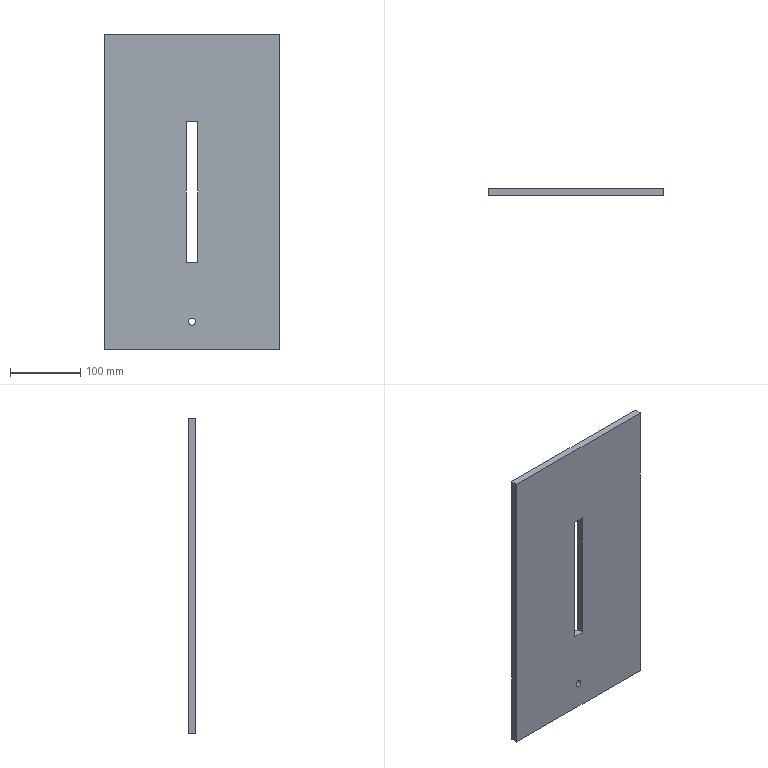Part | STEP file | tieqianjijia2 | 1 solid | 11 faces | box 250 x 10 x 450 mm | volume 1092215 mm3 | plane 10 | cylinder 1 | commonest cylinder face diameters 10 x1
STEP:
#1=CARTESIAN_POINT('',(0.,0.,0.));
#2=DIRECTION('',(0.,0.,1.));
#3=DIRECTION('',(1.,0.,0.));
#4=AXIS2_PLACEMENT_3D('',#1,#2,#3);
#5=CARTESIAN_POINT('',(0.,5.,-180.));
#6=VERTEX_POINT('',#5);
#7=CARTESIAN_POINT('',(0.,5.,-185.));
#8=DIRECTION('',(0.,1.,0.));
#9=DIRECTION('',(0.,0.,1.));
#10=AXIS2_PLACEMENT_3D('',#7,#8,#9);
#11=CIRCLE('',#10,5.);
#12=CARTESIAN_POINT('',(0.,5.,0.));
#13=DIRECTION('',(0.,1.,0.));
#14=DIRECTION('',(0.,0.,1.));
#15=AXIS2_PLACEMENT_3D('',#12,#13,#14);
#16=PLANE('',#15);
#17=CARTESIAN_POINT('',(-185.,0.));
#18=DIRECTION('',(1.,0.));
#19=AXIS2_PLACEMENT_2D('',#17,#18);
#20=CIRCLE('',#19,5.);
#21=(GEOMETRIC_REPRESENTATION_CONTEXT(2)PARAMETRIC_REPRESENTATION_CONTEXT()REPRESENTATION_CONTEXT('',''));
#22=DEFINITIONAL_REPRESENTATION('',(#20),#21);
#23=PCURVE('',#16,#22);
#24=CARTESIAN_POINT('',(0.,-5.,-185.));
#25=DIRECTION('',(0.,1.,0.));
#26=DIRECTION('',(0.,0.,1.));
#27=AXIS2_PLACEMENT_3D('',#24,#25,#26);
#28=CYLINDRICAL_SURFACE('',#27,5.);
#29=CARTESIAN_POINT('',(0.,10.));
#30=DIRECTION('',(1.,0.));
#31=VECTOR('',#30,1.);
#32=LINE('',#29,#31);
#33=(GEOMETRIC_REPRESENTATION_CONTEXT(2)PARAMETRIC_REPRESENTATION_CONTEXT()REPRESENTATION_CONTEXT('',''));
#34=DEFINITIONAL_REPRESENTATION('',(#32),#33);
#35=PCURVE('',#28,#34);
#36=SURFACE_CURVE('',#11,(#23,#35),.PCURVE_S1.);
#37=EDGE_CURVE('',#6,#6,#36,.T.);
#38=ORIENTED_EDGE('',*,*,#37,.F.);
#39=EDGE_LOOP('',(#38));
#40=FACE_BOUND('',#39,.T.);
#41=CARTESIAN_POINT('',(125.,5.,225.));
#42=VERTEX_POINT('',#41);
#43=CARTESIAN_POINT('',(125.,5.,-225.));
#44=VERTEX_POINT('',#43);
#45=CARTESIAN_POINT('',(125.,5.,-225.));
#46=DIRECTION('',(0.,0.,-1.));
#47=VECTOR('',#46,1.);
#48=LINE('',#45,#47);
#49=CARTESIAN_POINT('',(-225.,125.));
#50=DIRECTION('',(-1.,0.));
#51=VECTOR('',#50,1.);
#52=LINE('',#49,#51);
#53=(GEOMETRIC_REPRESENTATION_CONTEXT(2)PARAMETRIC_REPRESENTATION_CONTEXT()REPRESENTATION_CONTEXT('',''));
#54=DEFINITIONAL_REPRESENTATION('',(#52),#53);
#55=PCURVE('',#16,#54);
#56=CARTESIAN_POINT('',(125.,5.,-225.));
#57=DIRECTION('',(-1.,0.,0.));
#58=DIRECTION('',(0.,0.,1.));
#59=AXIS2_PLACEMENT_3D('',#56,#57,#58);
#60=PLANE('',#59);
#61=CARTESIAN_POINT('',(0.,0.));
#62=DIRECTION('',(-1.,0.));
#63=VECTOR('',#62,1.);
#64=LINE('',#61,#63);
#65=(GEOMETRIC_REPRESENTATION_CONTEXT(2)PARAMETRIC_REPRESENTATION_CONTEXT()REPRESENTATION_CONTEXT('',''));
#66=DEFINITIONAL_REPRESENTATION('',(#64),#65);
#67=PCURVE('',#60,#66);
#68=SURFACE_CURVE('',#48,(#55,#67),.PCURVE_S1.);
#69=EDGE_CURVE('',#42,#44,#68,.T.);
#70=ORIENTED_EDGE('',*,*,#69,.T.);
#71=CARTESIAN_POINT('',(-125.,5.,-225.));
#72=VERTEX_POINT('',#71);
#73=CARTESIAN_POINT('',(-125.,5.,-225.));
#74=DIRECTION('',(-1.,0.,0.));
#75=VECTOR('',#74,1.);
#76=LINE('',#73,#75);
#77=CARTESIAN_POINT('',(-225.,-125.));
#78=DIRECTION('',(0.,-1.));
#79=VECTOR('',#78,1.);
#80=LINE('',#77,#79);
#81=(GEOMETRIC_REPRESENTATION_CONTEXT(2)PARAMETRIC_REPRESENTATION_CONTEXT()REPRESENTATION_CONTEXT('',''));
#82=DEFINITIONAL_REPRESENTATION('',(#80),#81);
#83=PCURVE('',#16,#82);
#84=CARTESIAN_POINT('',(-125.,5.,-225.));
#85=DIRECTION('',(0.,0.,1.));
#86=DIRECTION('',(1.,0.,0.));
#87=AXIS2_PLACEMENT_3D('',#84,#85,#86);
#88=PLANE('',#87);
#89=CARTESIAN_POINT('',(0.,0.));
#90=DIRECTION('',(-1.,0.));
#91=VECTOR('',#90,1.);
#92=LINE('',#89,#91);
#93=(GEOMETRIC_REPRESENTATION_CONTEXT(2)PARAMETRIC_REPRESENTATION_CONTEXT()REPRESENTATION_CONTEXT('',''));
#94=DEFINITIONAL_REPRESENTATION('',(#92),#93);
#95=PCURVE('',#88,#94);
#96=SURFACE_CURVE('',#76,(#83,#95),.PCURVE_S1.);
#97=EDGE_CURVE('',#44,#72,#96,.T.);
#98=ORIENTED_EDGE('',*,*,#97,.T.);
#99=CARTESIAN_POINT('',(-125.,5.,225.));
#100=VERTEX_POINT('',#99);
#101=CARTESIAN_POINT('',(-125.,5.,-225.));
#102=DIRECTION('',(0.,0.,1.));
#103=VECTOR('',#102,1.);
#104=LINE('',#101,#103);
#105=CARTESIAN_POINT('',(-225.,-125.));
#106=DIRECTION('',(1.,0.));
#107=VECTOR('',#106,1.);
#108=LINE('',#105,#107);
#109=(GEOMETRIC_REPRESENTATION_CONTEXT(2)PARAMETRIC_REPRESENTATION_CONTEXT()REPRESENTATION_CONTEXT('',''));
#110=DEFINITIONAL_REPRESENTATION('',(#108),#109);
#111=PCURVE('',#16,#110);
#112=CARTESIAN_POINT('',(-125.,5.,-225.));
#113=DIRECTION('',(1.,0.,0.));
#114=DIRECTION('',(0.,0.,-1.));
#115=AXIS2_PLACEMENT_3D('',#112,#113,#114);
#116=PLANE('',#115);
#117=CARTESIAN_POINT('',(0.,0.));
#118=DIRECTION('',(-1.,0.));
#119=VECTOR('',#118,1.);
#120=LINE('',#117,#119);
#121=(GEOMETRIC_REPRESENTATION_CONTEXT(2)PARAMETRIC_REPRESENTATION_CONTEXT()REPRESENTATION_CONTEXT('',''));
#122=DEFINITIONAL_REPRESENTATION('',(#120),#121);
#123=PCURVE('',#116,#122);
#124=SURFACE_CURVE('',#104,(#111,#123),.PCURVE_S1.);
#125=EDGE_CURVE('',#72,#100,#124,.T.);
#126=ORIENTED_EDGE('',*,*,#125,.T.);
#127=CARTESIAN_POINT('',(-125.,5.,225.));
#128=DIRECTION('',(1.,0.,0.));
#129=VECTOR('',#128,1.);
#130=LINE('',#127,#129);
#131=CARTESIAN_POINT('',(225.,-125.));
#132=DIRECTION('',(0.,1.));
#133=VECTOR('',#132,1.);
#134=LINE('',#131,#133);
#135=(GEOMETRIC_REPRESENTATION_CONTEXT(2)PARAMETRIC_REPRESENTATION_CONTEXT()REPRESENTATION_CONTEXT('',''));
#136=DEFINITIONAL_REPRESENTATION('',(#134),#135);
#137=PCURVE('',#16,#136);
#138=CARTESIAN_POINT('',(-125.,5.,225.));
#139=DIRECTION('',(0.,0.,-1.));
#140=DIRECTION('',(-1.,0.,0.));
#141=AXIS2_PLACEMENT_3D('',#138,#139,#140);
#142=PLANE('',#141);
#143=CARTESIAN_POINT('',(0.,0.));
#144=DIRECTION('',(-1.,0.));
#145=VECTOR('',#144,1.);
#146=LINE('',#143,#145);
#147=(GEOMETRIC_REPRESENTATION_CONTEXT(2)PARAMETRIC_REPRESENTATION_CONTEXT()REPRESENTATION_CONTEXT('',''));
#148=DEFINITIONAL_REPRESENTATION('',(#146),#147);
#149=PCURVE('',#142,#148);
#150=SURFACE_CURVE('',#130,(#137,#149),.PCURVE_S1.);
#151=EDGE_CURVE('',#100,#42,#150,.T.);
#152=ORIENTED_EDGE('',*,*,#151,.T.);
#153=EDGE_LOOP('',(#70,#98,#126,#152));
#154=FACE_BOUND('',#153,.T.);
#155=CARTESIAN_POINT('',(-8.,5.,-100.));
#156=VERTEX_POINT('',#155);
#157=CARTESIAN_POINT('',(-8.,5.,100.));
#158=VERTEX_POINT('',#157);
#159=CARTESIAN_POINT('',(-8.,5.,-100.));
#160=DIRECTION('',(0.,0.,1.));
#161=VECTOR('',#160,1.);
#162=LINE('',#159,#161);
#163=CARTESIAN_POINT('',(-100.,-8.));
#164=DIRECTION('',(1.,0.));
#165=VECTOR('',#164,1.);
#166=LINE('',#163,#165);
#167=(GEOMETRIC_REPRESENTATION_CONTEXT(2)PARAMETRIC_REPRESENTATION_CONTEXT()REPRESENTATION_CONTEXT('',''));
#168=DEFINITIONAL_REPRESENTATION('',(#166),#167);
#169=PCURVE('',#16,#168);
#170=CARTESIAN_POINT('',(-8.,-5.,-100.));
#171=DIRECTION('',(-1.,0.,0.));
#172=DIRECTION('',(0.,0.,1.));
#173=AXIS2_PLACEMENT_3D('',#170,#171,#172);
#174=PLANE('',#173);
#175=CARTESIAN_POINT('',(0.,10.));
#176=DIRECTION('',(1.,0.));
#177=VECTOR('',#176,1.);
#178=LINE('',#175,#177);
#179=(GEOMETRIC_REPRESENTATION_CONTEXT(2)PARAMETRIC_REPRESENTATION_CONTEXT()REPRESENTATION_CONTEXT('',''));
#180=DEFINITIONAL_REPRESENTATION('',(#178),#179);
#181=PCURVE('',#174,#180);
#182=SURFACE_CURVE('',#162,(#169,#181),.PCURVE_S1.);
#183=EDGE_CURVE('',#156,#158,#182,.T.);
#184=ORIENTED_EDGE('',*,*,#183,.F.);
#185=CARTESIAN_POINT('',(8.,5.,-100.));
#186=VERTEX_POINT('',#185);
#187=CARTESIAN_POINT('',(-8.,5.,-100.));
#188=DIRECTION('',(1.,0.,0.));
#189=VECTOR('',#188,1.);
#190=LINE('',#187,#189);
#191=CARTESIAN_POINT('',(-100.,-8.));
#192=DIRECTION('',(0.,1.));
#193=VECTOR('',#192,1.);
#194=LINE('',#191,#193);
#195=(GEOMETRIC_REPRESENTATION_CONTEXT(2)PARAMETRIC_REPRESENTATION_CONTEXT()REPRESENTATION_CONTEXT('',''));
#196=DEFINITIONAL_REPRESENTATION('',(#194),#195);
#197=PCURVE('',#16,#196);
#198=CARTESIAN_POINT('',(-8.,-5.,-100.));
#199=DIRECTION('',(0.,0.,1.));
#200=DIRECTION('',(1.,0.,0.));
#201=AXIS2_PLACEMENT_3D('',#198,#199,#200);
#202=PLANE('',#201);
#203=CARTESIAN_POINT('',(0.,10.));
#204=DIRECTION('',(1.,0.));
#205=VECTOR('',#204,1.);
#206=LINE('',#203,#205);
#207=(GEOMETRIC_REPRESENTATION_CONTEXT(2)PARAMETRIC_REPRESENTATION_CONTEXT()REPRESENTATION_CONTEXT('',''));
#208=DEFINITIONAL_REPRESENTATION('',(#206),#207);
#209=PCURVE('',#202,#208);
#210=SURFACE_CURVE('',#190,(#197,#209),.PCURVE_S1.);
#211=EDGE_CURVE('',#156,#186,#210,.T.);
#212=ORIENTED_EDGE('',*,*,#211,.T.);
#213=CARTESIAN_POINT('',(8.,5.,100.));
#214=VERTEX_POINT('',#213);
#215=CARTESIAN_POINT('',(8.,5.,100.));
#216=DIRECTION('',(0.,0.,-1.));
#217=VECTOR('',#216,1.);
#218=LINE('',#215,#217);
#219=CARTESIAN_POINT('',(100.,8.));
#220=DIRECTION('',(-1.,0.));
#221=VECTOR('',#220,1.);
#222=LINE('',#219,#221);
#223=(GEOMETRIC_REPRESENTATION_CONTEXT(2)PARAMETRIC_REPRESENTATION_CONTEXT()REPRESENTATION_CONTEXT('',''));
#224=DEFINITIONAL_REPRESENTATION('',(#222),#223);
#225=PCURVE('',#16,#224);
#226=CARTESIAN_POINT('',(8.,-5.,100.));
#227=DIRECTION('',(1.,0.,0.));
#228=DIRECTION('',(0.,0.,-1.));
#229=AXIS2_PLACEMENT_3D('',#226,#227,#228);
#230=PLANE('',#229);
#231=CARTESIAN_POINT('',(0.,10.));
#232=DIRECTION('',(1.,0.));
#233=VECTOR('',#232,1.);
#234=LINE('',#231,#233);
#235=(GEOMETRIC_REPRESENTATION_CONTEXT(2)PARAMETRIC_REPRESENTATION_CONTEXT()REPRESENTATION_CONTEXT('',''));
#236=DEFINITIONAL_REPRESENTATION('',(#234),#235);
#237=PCURVE('',#230,#236);
#238=SURFACE_CURVE('',#218,(#225,#237),.PCURVE_S1.);
#239=EDGE_CURVE('',#214,#186,#238,.T.);
#240=ORIENTED_EDGE('',*,*,#239,.F.);
#241=CARTESIAN_POINT('',(-8.,5.,100.));
#242=DIRECTION('',(1.,0.,0.));
#243=VECTOR('',#242,1.);
#244=LINE('',#241,#243);
#245=CARTESIAN_POINT('',(100.,-8.));
#246=DIRECTION('',(0.,1.));
#247=VECTOR('',#246,1.);
#248=LINE('',#245,#247);
#249=(GEOMETRIC_REPRESENTATION_CONTEXT(2)PARAMETRIC_REPRESENTATION_CONTEXT()REPRESENTATION_CONTEXT('',''));
#250=DEFINITIONAL_REPRESENTATION('',(#248),#249);
#251=PCURVE('',#16,#250);
#252=CARTESIAN_POINT('',(-8.,-5.,100.));
#253=DIRECTION('',(0.,0.,1.));
#254=DIRECTION('',(1.,0.,0.));
#255=AXIS2_PLACEMENT_3D('',#252,#253,#254);
#256=PLANE('',#255);
#257=CARTESIAN_POINT('',(0.,10.));
#258=DIRECTION('',(1.,0.));
#259=VECTOR('',#258,1.);
#260=LINE('',#257,#259);
#261=(GEOMETRIC_REPRESENTATION_CONTEXT(2)PARAMETRIC_REPRESENTATION_CONTEXT()REPRESENTATION_CONTEXT('',''));
#262=DEFINITIONAL_REPRESENTATION('',(#260),#261);
#263=PCURVE('',#256,#262);
#264=SURFACE_CURVE('',#244,(#251,#263),.PCURVE_S1.);
#265=EDGE_CURVE('',#158,#214,#264,.T.);
#266=ORIENTED_EDGE('',*,*,#265,.F.);
#267=EDGE_LOOP('',(#184,#212,#240,#266));
#268=FACE_BOUND('',#267,.T.);
#269=ADVANCED_FACE('',(#40,#154,#268),#16,.T.);
#270=CARTESIAN_POINT('',(0.,-5.,-180.));
#271=VERTEX_POINT('',#270);
#272=CARTESIAN_POINT('',(0.,-5.,-185.));
#273=DIRECTION('',(0.,1.,0.));
#274=DIRECTION('',(0.,0.,1.));
#275=AXIS2_PLACEMENT_3D('',#272,#273,#274);
#276=CIRCLE('',#275,5.);
#277=CARTESIAN_POINT('',(0.,-5.,0.));
#278=DIRECTION('',(0.,1.,0.));
#279=DIRECTION('',(0.,0.,1.));
#280=AXIS2_PLACEMENT_3D('',#277,#278,#279);
#281=PLANE('',#280);
#282=CARTESIAN_POINT('',(-185.,0.));
#283=DIRECTION('',(1.,0.));
#284=AXIS2_PLACEMENT_2D('',#282,#283);
#285=CIRCLE('',#284,5.);
#286=(GEOMETRIC_REPRESENTATION_CONTEXT(2)PARAMETRIC_REPRESENTATION_CONTEXT()REPRESENTATION_CONTEXT('',''));
#287=DEFINITIONAL_REPRESENTATION('',(#285),#286);
#288=PCURVE('',#281,#287);
#289=CARTESIAN_POINT('',(0.,0.));
#290=DIRECTION('',(1.,0.));
#291=VECTOR('',#290,1.);
#292=LINE('',#289,#291);
#293=(GEOMETRIC_REPRESENTATION_CONTEXT(2)PARAMETRIC_REPRESENTATION_CONTEXT()REPRESENTATION_CONTEXT('',''));
#294=DEFINITIONAL_REPRESENTATION('',(#292),#293);
#295=PCURVE('',#28,#294);
#296=SURFACE_CURVE('',#276,(#288,#295),.PCURVE_S1.);
#297=EDGE_CURVE('',#271,#271,#296,.T.);
#298=ORIENTED_EDGE('',*,*,#297,.T.);
#299=EDGE_LOOP('',(#298));
#300=FACE_BOUND('',#299,.T.);
#301=CARTESIAN_POINT('',(125.,-5.,225.));
#302=VERTEX_POINT('',#301);
#303=CARTESIAN_POINT('',(125.,-5.,-225.));
#304=VERTEX_POINT('',#303);
#305=CARTESIAN_POINT('',(125.,-5.,-225.));
#306=DIRECTION('',(0.,0.,-1.));
#307=VECTOR('',#306,1.);
#308=LINE('',#305,#307);
#309=CARTESIAN_POINT('',(-225.,125.));
#310=DIRECTION('',(-1.,0.));
#311=VECTOR('',#310,1.);
#312=LINE('',#309,#311);
#313=(GEOMETRIC_REPRESENTATION_CONTEXT(2)PARAMETRIC_REPRESENTATION_CONTEXT()REPRESENTATION_CONTEXT('',''));
#314=DEFINITIONAL_REPRESENTATION('',(#312),#313);
#315=PCURVE('',#281,#314);
#316=CARTESIAN_POINT('',(0.,-10.));
#317=DIRECTION('',(-1.,0.));
#318=VECTOR('',#317,1.);
#319=LINE('',#316,#318);
#320=(GEOMETRIC_REPRESENTATION_CONTEXT(2)PARAMETRIC_REPRESENTATION_CONTEXT()REPRESENTATION_CONTEXT('',''));
#321=DEFINITIONAL_REPRESENTATION('',(#319),#320);
#322=PCURVE('',#60,#321);
#323=SURFACE_CURVE('',#308,(#315,#322),.PCURVE_S1.);
#324=EDGE_CURVE('',#302,#304,#323,.T.);
#325=ORIENTED_EDGE('',*,*,#324,.F.);
#326=CARTESIAN_POINT('',(-125.,-5.,225.));
#327=VERTEX_POINT('',#326);
#328=CARTESIAN_POINT('',(-125.,-5.,225.));
#329=DIRECTION('',(1.,0.,0.));
#330=VECTOR('',#329,1.);
#331=LINE('',#328,#330);
#332=CARTESIAN_POINT('',(225.,-125.));
#333=DIRECTION('',(0.,1.));
#334=VECTOR('',#333,1.);
#335=LINE('',#332,#334);
#336=(GEOMETRIC_REPRESENTATION_CONTEXT(2)PARAMETRIC_REPRESENTATION_CONTEXT()REPRESENTATION_CONTEXT('',''));
#337=DEFINITIONAL_REPRESENTATION('',(#335),#336);
#338=PCURVE('',#281,#337);
#339=CARTESIAN_POINT('',(0.,-10.));
#340=DIRECTION('',(-1.,0.));
#341=VECTOR('',#340,1.);
#342=LINE('',#339,#341);
#343=(GEOMETRIC_REPRESENTATION_CONTEXT(2)PARAMETRIC_REPRESENTATION_CONTEXT()REPRESENTATION_CONTEXT('',''));
#344=DEFINITIONAL_REPRESENTATION('',(#342),#343);
#345=PCURVE('',#142,#344);
#346=SURFACE_CURVE('',#331,(#338,#345),.PCURVE_S1.);
#347=EDGE_CURVE('',#327,#302,#346,.T.);
#348=ORIENTED_EDGE('',*,*,#347,.F.);
#349=CARTESIAN_POINT('',(-125.,-5.,-225.));
#350=VERTEX_POINT('',#349);
#351=CARTESIAN_POINT('',(-125.,-5.,-225.));
#352=DIRECTION('',(0.,0.,1.));
#353=VECTOR('',#352,1.);
#354=LINE('',#351,#353);
#355=CARTESIAN_POINT('',(-225.,-125.));
#356=DIRECTION('',(1.,0.));
#357=VECTOR('',#356,1.);
#358=LINE('',#355,#357);
#359=(GEOMETRIC_REPRESENTATION_CONTEXT(2)PARAMETRIC_REPRESENTATION_CONTEXT()REPRESENTATION_CONTEXT('',''));
#360=DEFINITIONAL_REPRESENTATION('',(#358),#359);
#361=PCURVE('',#281,#360);
#362=CARTESIAN_POINT('',(0.,-10.));
#363=DIRECTION('',(-1.,0.));
#364=VECTOR('',#363,1.);
#365=LINE('',#362,#364);
#366=(GEOMETRIC_REPRESENTATION_CONTEXT(2)PARAMETRIC_REPRESENTATION_CONTEXT()REPRESENTATION_CONTEXT('',''));
#367=DEFINITIONAL_REPRESENTATION('',(#365),#366);
#368=PCURVE('',#116,#367);
#369=SURFACE_CURVE('',#354,(#361,#368),.PCURVE_S1.);
#370=EDGE_CURVE('',#350,#327,#369,.T.);
#371=ORIENTED_EDGE('',*,*,#370,.F.);
#372=CARTESIAN_POINT('',(-125.,-5.,-225.));
#373=DIRECTION('',(-1.,0.,0.));
#374=VECTOR('',#373,1.);
#375=LINE('',#372,#374);
#376=CARTESIAN_POINT('',(-225.,-125.));
#377=DIRECTION('',(0.,-1.));
#378=VECTOR('',#377,1.);
#379=LINE('',#376,#378);
#380=(GEOMETRIC_REPRESENTATION_CONTEXT(2)PARAMETRIC_REPRESENTATION_CONTEXT()REPRESENTATION_CONTEXT('',''));
#381=DEFINITIONAL_REPRESENTATION('',(#379),#380);
#382=PCURVE('',#281,#381);
#383=CARTESIAN_POINT('',(0.,-10.));
#384=DIRECTION('',(-1.,0.));
#385=VECTOR('',#384,1.);
#386=LINE('',#383,#385);
#387=(GEOMETRIC_REPRESENTATION_CONTEXT(2)PARAMETRIC_REPRESENTATION_CONTEXT()REPRESENTATION_CONTEXT('',''));
#388=DEFINITIONAL_REPRESENTATION('',(#386),#387);
#389=PCURVE('',#88,#388);
#390=SURFACE_CURVE('',#375,(#382,#389),.PCURVE_S1.);
#391=EDGE_CURVE('',#304,#350,#390,.T.);
#392=ORIENTED_EDGE('',*,*,#391,.F.);
#393=EDGE_LOOP('',(#325,#348,#371,#392));
#394=FACE_BOUND('',#393,.T.);
#395=CARTESIAN_POINT('',(-8.,-5.,-100.));
#396=VERTEX_POINT('',#395);
#397=CARTESIAN_POINT('',(8.,-5.,-100.));
#398=VERTEX_POINT('',#397);
#399=CARTESIAN_POINT('',(-8.,-5.,-100.));
#400=DIRECTION('',(1.,0.,0.));
#401=VECTOR('',#400,1.);
#402=LINE('',#399,#401);
#403=CARTESIAN_POINT('',(-100.,-8.));
#404=DIRECTION('',(0.,1.));
#405=VECTOR('',#404,1.);
#406=LINE('',#403,#405);
#407=(GEOMETRIC_REPRESENTATION_CONTEXT(2)PARAMETRIC_REPRESENTATION_CONTEXT()REPRESENTATION_CONTEXT('',''));
#408=DEFINITIONAL_REPRESENTATION('',(#406),#407);
#409=PCURVE('',#281,#408);
#410=CARTESIAN_POINT('',(0.,0.));
#411=DIRECTION('',(1.,0.));
#412=VECTOR('',#411,1.);
#413=LINE('',#410,#412);
#414=(GEOMETRIC_REPRESENTATION_CONTEXT(2)PARAMETRIC_REPRESENTATION_CONTEXT()REPRESENTATION_CONTEXT('',''));
#415=DEFINITIONAL_REPRESENTATION('',(#413),#414);
#416=PCURVE('',#202,#415);
#417=SURFACE_CURVE('',#402,(#409,#416),.PCURVE_S1.);
#418=EDGE_CURVE('',#396,#398,#417,.T.);
#419=ORIENTED_EDGE('',*,*,#418,.F.);
#420=CARTESIAN_POINT('',(-8.,-5.,100.));
#421=VERTEX_POINT('',#420);
#422=CARTESIAN_POINT('',(-8.,-5.,-100.));
#423=DIRECTION('',(0.,0.,1.));
#424=VECTOR('',#423,1.);
#425=LINE('',#422,#424);
#426=CARTESIAN_POINT('',(-100.,-8.));
#427=DIRECTION('',(1.,0.));
#428=VECTOR('',#427,1.);
#429=LINE('',#426,#428);
#430=(GEOMETRIC_REPRESENTATION_CONTEXT(2)PARAMETRIC_REPRESENTATION_CONTEXT()REPRESENTATION_CONTEXT('',''));
#431=DEFINITIONAL_REPRESENTATION('',(#429),#430);
#432=PCURVE('',#281,#431);
#433=CARTESIAN_POINT('',(0.,0.));
#434=DIRECTION('',(1.,0.));
#435=VECTOR('',#434,1.);
#436=LINE('',#433,#435);
#437=(GEOMETRIC_REPRESENTATION_CONTEXT(2)PARAMETRIC_REPRESENTATION_CONTEXT()REPRESENTATION_CONTEXT('',''));
#438=DEFINITIONAL_REPRESENTATION('',(#436),#437);
#439=PCURVE('',#174,#438);
#440=SURFACE_CURVE('',#425,(#432,#439),.PCURVE_S1.);
#441=EDGE_CURVE('',#396,#421,#440,.T.);
#442=ORIENTED_EDGE('',*,*,#441,.T.);
#443=CARTESIAN_POINT('',(8.,-5.,100.));
#444=VERTEX_POINT('',#443);
#445=CARTESIAN_POINT('',(-8.,-5.,100.));
#446=DIRECTION('',(1.,0.,0.));
#447=VECTOR('',#446,1.);
#448=LINE('',#445,#447);
#449=CARTESIAN_POINT('',(100.,-8.));
#450=DIRECTION('',(0.,1.));
#451=VECTOR('',#450,1.);
#452=LINE('',#449,#451);
#453=(GEOMETRIC_REPRESENTATION_CONTEXT(2)PARAMETRIC_REPRESENTATION_CONTEXT()REPRESENTATION_CONTEXT('',''));
#454=DEFINITIONAL_REPRESENTATION('',(#452),#453);
#455=PCURVE('',#281,#454);
#456=CARTESIAN_POINT('',(0.,0.));
#457=DIRECTION('',(1.,0.));
#458=VECTOR('',#457,1.);
#459=LINE('',#456,#458);
#460=(GEOMETRIC_REPRESENTATION_CONTEXT(2)PARAMETRIC_REPRESENTATION_CONTEXT()REPRESENTATION_CONTEXT('',''));
#461=DEFINITIONAL_REPRESENTATION('',(#459),#460);
#462=PCURVE('',#256,#461);
#463=SURFACE_CURVE('',#448,(#455,#462),.PCURVE_S1.);
#464=EDGE_CURVE('',#421,#444,#463,.T.);
#465=ORIENTED_EDGE('',*,*,#464,.T.);
#466=CARTESIAN_POINT('',(8.,-5.,100.));
#467=DIRECTION('',(0.,0.,-1.));
#468=VECTOR('',#467,1.);
#469=LINE('',#466,#468);
#470=CARTESIAN_POINT('',(100.,8.));
#471=DIRECTION('',(-1.,0.));
#472=VECTOR('',#471,1.);
#473=LINE('',#470,#472);
#474=(GEOMETRIC_REPRESENTATION_CONTEXT(2)PARAMETRIC_REPRESENTATION_CONTEXT()REPRESENTATION_CONTEXT('',''));
#475=DEFINITIONAL_REPRESENTATION('',(#473),#474);
#476=PCURVE('',#281,#475);
#477=CARTESIAN_POINT('',(0.,0.));
#478=DIRECTION('',(1.,0.));
#479=VECTOR('',#478,1.);
#480=LINE('',#477,#479);
#481=(GEOMETRIC_REPRESENTATION_CONTEXT(2)PARAMETRIC_REPRESENTATION_CONTEXT()REPRESENTATION_CONTEXT('',''));
#482=DEFINITIONAL_REPRESENTATION('',(#480),#481);
#483=PCURVE('',#230,#482);
#484=SURFACE_CURVE('',#469,(#476,#483),.PCURVE_S1.);
#485=EDGE_CURVE('',#444,#398,#484,.T.);
#486=ORIENTED_EDGE('',*,*,#485,.T.);
#487=EDGE_LOOP('',(#419,#442,#465,#486));
#488=FACE_BOUND('',#487,.T.);
#489=ADVANCED_FACE('',(#300,#394,#488),#281,.F.);
#490=ORIENTED_EDGE('',*,*,#324,.T.);
#491=CARTESIAN_POINT('',(125.,5.,-225.));
#492=DIRECTION('',(0.,-1.,0.));
#493=VECTOR('',#492,1.);
#494=LINE('',#491,#493);
#495=CARTESIAN_POINT('',(0.,0.));
#496=DIRECTION('',(0.,-1.));
#497=VECTOR('',#496,1.);
#498=LINE('',#495,#497);
#499=(GEOMETRIC_REPRESENTATION_CONTEXT(2)PARAMETRIC_REPRESENTATION_CONTEXT()REPRESENTATION_CONTEXT('',''));
#500=DEFINITIONAL_REPRESENTATION('',(#498),#499);
#501=PCURVE('',#60,#500);
#502=CARTESIAN_POINT('',(250.,0.));
#503=DIRECTION('',(0.,-1.));
#504=VECTOR('',#503,1.);
#505=LINE('',#502,#504);
#506=(GEOMETRIC_REPRESENTATION_CONTEXT(2)PARAMETRIC_REPRESENTATION_CONTEXT()REPRESENTATION_CONTEXT('',''));
#507=DEFINITIONAL_REPRESENTATION('',(#505),#506);
#508=PCURVE('',#88,#507);
#509=SURFACE_CURVE('',#494,(#501,#508),.PCURVE_S1.);
#510=EDGE_CURVE('',#44,#304,#509,.T.);
#511=ORIENTED_EDGE('',*,*,#510,.F.);
#512=ORIENTED_EDGE('',*,*,#69,.F.);
#513=CARTESIAN_POINT('',(125.,5.,225.));
#514=DIRECTION('',(0.,-1.,0.));
#515=VECTOR('',#514,1.);
#516=LINE('',#513,#515);
#517=CARTESIAN_POINT('',(450.,0.));
#518=DIRECTION('',(0.,-1.));
#519=VECTOR('',#518,1.);
#520=LINE('',#517,#519);
#521=(GEOMETRIC_REPRESENTATION_CONTEXT(2)PARAMETRIC_REPRESENTATION_CONTEXT()REPRESENTATION_CONTEXT('',''));
#522=DEFINITIONAL_REPRESENTATION('',(#520),#521);
#523=PCURVE('',#60,#522);
#524=CARTESIAN_POINT('',(-250.,0.));
#525=DIRECTION('',(0.,-1.));
#526=VECTOR('',#525,1.);
#527=LINE('',#524,#526);
#528=(GEOMETRIC_REPRESENTATION_CONTEXT(2)PARAMETRIC_REPRESENTATION_CONTEXT()REPRESENTATION_CONTEXT('',''));
#529=DEFINITIONAL_REPRESENTATION('',(#527),#528);
#530=PCURVE('',#142,#529);
#531=SURFACE_CURVE('',#516,(#523,#530),.PCURVE_S1.);
#532=EDGE_CURVE('',#42,#302,#531,.T.);
#533=ORIENTED_EDGE('',*,*,#532,.T.);
#534=EDGE_LOOP('',(#490,#511,#512,#533));
#535=FACE_BOUND('',#534,.T.);
#536=ADVANCED_FACE('',(#535),#60,.F.);
#537=ORIENTED_EDGE('',*,*,#391,.T.);
#538=CARTESIAN_POINT('',(-125.,5.,-225.));
#539=DIRECTION('',(0.,-1.,0.));
#540=VECTOR('',#539,1.);
#541=LINE('',#538,#540);
#542=CARTESIAN_POINT('',(0.,0.));
#543=DIRECTION('',(0.,-1.));
#544=VECTOR('',#543,1.);
#545=LINE('',#542,#544);
#546=(GEOMETRIC_REPRESENTATION_CONTEXT(2)PARAMETRIC_REPRESENTATION_CONTEXT()REPRESENTATION_CONTEXT('',''));
#547=DEFINITIONAL_REPRESENTATION('',(#545),#546);
#548=PCURVE('',#88,#547);
#549=CARTESIAN_POINT('',(0.,0.));
#550=DIRECTION('',(0.,-1.));
#551=VECTOR('',#550,1.);
#552=LINE('',#549,#551);
#553=(GEOMETRIC_REPRESENTATION_CONTEXT(2)PARAMETRIC_REPRESENTATION_CONTEXT()REPRESENTATION_CONTEXT('',''));
#554=DEFINITIONAL_REPRESENTATION('',(#552),#553);
#555=PCURVE('',#116,#554);
#556=SURFACE_CURVE('',#541,(#548,#555),.PCURVE_S1.);
#557=EDGE_CURVE('',#72,#350,#556,.T.);
#558=ORIENTED_EDGE('',*,*,#557,.F.);
#559=ORIENTED_EDGE('',*,*,#97,.F.);
#560=ORIENTED_EDGE('',*,*,#510,.T.);
#561=EDGE_LOOP('',(#537,#558,#559,#560));
#562=FACE_BOUND('',#561,.T.);
#563=ADVANCED_FACE('',(#562),#88,.F.);
#564=ORIENTED_EDGE('',*,*,#370,.T.);
#565=CARTESIAN_POINT('',(-125.,5.,225.));
#566=DIRECTION('',(0.,-1.,0.));
#567=VECTOR('',#566,1.);
#568=LINE('',#565,#567);
#569=CARTESIAN_POINT('',(-450.,0.));
#570=DIRECTION('',(0.,-1.));
#571=VECTOR('',#570,1.);
#572=LINE('',#569,#571);
#573=(GEOMETRIC_REPRESENTATION_CONTEXT(2)PARAMETRIC_REPRESENTATION_CONTEXT()REPRESENTATION_CONTEXT('',''));
#574=DEFINITIONAL_REPRESENTATION('',(#572),#573);
#575=PCURVE('',#116,#574);
#576=CARTESIAN_POINT('',(0.,0.));
#577=DIRECTION('',(0.,-1.));
#578=VECTOR('',#577,1.);
#579=LINE('',#576,#578);
#580=(GEOMETRIC_REPRESENTATION_CONTEXT(2)PARAMETRIC_REPRESENTATION_CONTEXT()REPRESENTATION_CONTEXT('',''));
#581=DEFINITIONAL_REPRESENTATION('',(#579),#580);
#582=PCURVE('',#142,#581);
#583=SURFACE_CURVE('',#568,(#575,#582),.PCURVE_S1.);
#584=EDGE_CURVE('',#100,#327,#583,.T.);
#585=ORIENTED_EDGE('',*,*,#584,.F.);
#586=ORIENTED_EDGE('',*,*,#125,.F.);
#587=ORIENTED_EDGE('',*,*,#557,.T.);
#588=EDGE_LOOP('',(#564,#585,#586,#587));
#589=FACE_BOUND('',#588,.T.);
#590=ADVANCED_FACE('',(#589),#116,.F.);
#591=ORIENTED_EDGE('',*,*,#347,.T.);
#592=ORIENTED_EDGE('',*,*,#532,.F.);
#593=ORIENTED_EDGE('',*,*,#151,.F.);
#594=ORIENTED_EDGE('',*,*,#584,.T.);
#595=EDGE_LOOP('',(#591,#592,#593,#594));
#596=FACE_BOUND('',#595,.T.);
#597=ADVANCED_FACE('',(#596),#142,.F.);
#598=ORIENTED_EDGE('',*,*,#211,.F.);
#599=CARTESIAN_POINT('',(-8.,-5.,-100.));
#600=DIRECTION('',(0.,1.,0.));
#601=VECTOR('',#600,1.);
#602=LINE('',#599,#601);
#603=CARTESIAN_POINT('',(0.,0.));
#604=DIRECTION('',(0.,1.));
#605=VECTOR('',#604,1.);
#606=LINE('',#603,#605);
#607=(GEOMETRIC_REPRESENTATION_CONTEXT(2)PARAMETRIC_REPRESENTATION_CONTEXT()REPRESENTATION_CONTEXT('',''));
#608=DEFINITIONAL_REPRESENTATION('',(#606),#607);
#609=PCURVE('',#202,#608);
#610=CARTESIAN_POINT('',(0.,0.));
#611=DIRECTION('',(0.,1.));
#612=VECTOR('',#611,1.);
#613=LINE('',#610,#612);
#614=(GEOMETRIC_REPRESENTATION_CONTEXT(2)PARAMETRIC_REPRESENTATION_CONTEXT()REPRESENTATION_CONTEXT('',''));
#615=DEFINITIONAL_REPRESENTATION('',(#613),#614);
#616=PCURVE('',#174,#615);
#617=SURFACE_CURVE('',#602,(#609,#616),.PCURVE_S1.);
#618=EDGE_CURVE('',#396,#156,#617,.T.);
#619=ORIENTED_EDGE('',*,*,#618,.F.);
#620=ORIENTED_EDGE('',*,*,#418,.T.);
#621=CARTESIAN_POINT('',(8.,-5.,-100.));
#622=DIRECTION('',(0.,1.,0.));
#623=VECTOR('',#622,1.);
#624=LINE('',#621,#623);
#625=CARTESIAN_POINT('',(16.,0.));
#626=DIRECTION('',(0.,1.));
#627=VECTOR('',#626,1.);
#628=LINE('',#625,#627);
#629=(GEOMETRIC_REPRESENTATION_CONTEXT(2)PARAMETRIC_REPRESENTATION_CONTEXT()REPRESENTATION_CONTEXT('',''));
#630=DEFINITIONAL_REPRESENTATION('',(#628),#629);
#631=PCURVE('',#202,#630);
#632=CARTESIAN_POINT('',(200.,0.));
#633=DIRECTION('',(0.,1.));
#634=VECTOR('',#633,1.);
#635=LINE('',#632,#634);
#636=(GEOMETRIC_REPRESENTATION_CONTEXT(2)PARAMETRIC_REPRESENTATION_CONTEXT()REPRESENTATION_CONTEXT('',''));
#637=DEFINITIONAL_REPRESENTATION('',(#635),#636);
#638=PCURVE('',#230,#637);
#639=SURFACE_CURVE('',#624,(#631,#638),.PCURVE_S1.);
#640=EDGE_CURVE('',#398,#186,#639,.T.);
#641=ORIENTED_EDGE('',*,*,#640,.T.);
#642=EDGE_LOOP('',(#598,#619,#620,#641));
#643=FACE_BOUND('',#642,.T.);
#644=ADVANCED_FACE('',(#643),#202,.T.);
#645=ORIENTED_EDGE('',*,*,#239,.T.);
#646=ORIENTED_EDGE('',*,*,#640,.F.);
#647=ORIENTED_EDGE('',*,*,#485,.F.);
#648=CARTESIAN_POINT('',(8.,-5.,100.));
#649=DIRECTION('',(0.,1.,0.));
#650=VECTOR('',#649,1.);
#651=LINE('',#648,#650);
#652=CARTESIAN_POINT('',(0.,0.));
#653=DIRECTION('',(0.,1.));
#654=VECTOR('',#653,1.);
#655=LINE('',#652,#654);
#656=(GEOMETRIC_REPRESENTATION_CONTEXT(2)PARAMETRIC_REPRESENTATION_CONTEXT()REPRESENTATION_CONTEXT('',''));
#657=DEFINITIONAL_REPRESENTATION('',(#655),#656);
#658=PCURVE('',#230,#657);
#659=CARTESIAN_POINT('',(16.,0.));
#660=DIRECTION('',(0.,1.));
#661=VECTOR('',#660,1.);
#662=LINE('',#659,#661);
#663=(GEOMETRIC_REPRESENTATION_CONTEXT(2)PARAMETRIC_REPRESENTATION_CONTEXT()REPRESENTATION_CONTEXT('',''));
#664=DEFINITIONAL_REPRESENTATION('',(#662),#663);
#665=PCURVE('',#256,#664);
#666=SURFACE_CURVE('',#651,(#658,#665),.PCURVE_S1.);
#667=EDGE_CURVE('',#444,#214,#666,.T.);
#668=ORIENTED_EDGE('',*,*,#667,.T.);
#669=EDGE_LOOP('',(#645,#646,#647,#668));
#670=FACE_BOUND('',#669,.T.);
#671=ADVANCED_FACE('',(#670),#230,.F.);
#672=ORIENTED_EDGE('',*,*,#265,.T.);
#673=ORIENTED_EDGE('',*,*,#667,.F.);
#674=ORIENTED_EDGE('',*,*,#464,.F.);
#675=CARTESIAN_POINT('',(-8.,-5.,100.));
#676=DIRECTION('',(0.,1.,0.));
#677=VECTOR('',#676,1.);
#678=LINE('',#675,#677);
#679=CARTESIAN_POINT('',(0.,0.));
#680=DIRECTION('',(0.,1.));
#681=VECTOR('',#680,1.);
#682=LINE('',#679,#681);
#683=(GEOMETRIC_REPRESENTATION_CONTEXT(2)PARAMETRIC_REPRESENTATION_CONTEXT()REPRESENTATION_CONTEXT('',''));
#684=DEFINITIONAL_REPRESENTATION('',(#682),#683);
#685=PCURVE('',#256,#684);
#686=CARTESIAN_POINT('',(200.,0.));
#687=DIRECTION('',(0.,1.));
#688=VECTOR('',#687,1.);
#689=LINE('',#686,#688);
#690=(GEOMETRIC_REPRESENTATION_CONTEXT(2)PARAMETRIC_REPRESENTATION_CONTEXT()REPRESENTATION_CONTEXT('',''));
#691=DEFINITIONAL_REPRESENTATION('',(#689),#690);
#692=PCURVE('',#174,#691);
#693=SURFACE_CURVE('',#678,(#685,#692),.PCURVE_S1.);
#694=EDGE_CURVE('',#421,#158,#693,.T.);
#695=ORIENTED_EDGE('',*,*,#694,.T.);
#696=EDGE_LOOP('',(#672,#673,#674,#695));
#697=FACE_BOUND('',#696,.T.);
#698=ADVANCED_FACE('',(#697),#256,.F.);
#699=ORIENTED_EDGE('',*,*,#183,.T.);
#700=ORIENTED_EDGE('',*,*,#694,.F.);
#701=ORIENTED_EDGE('',*,*,#441,.F.);
#702=ORIENTED_EDGE('',*,*,#618,.T.);
#703=EDGE_LOOP('',(#699,#700,#701,#702));
#704=FACE_BOUND('',#703,.T.);
#705=ADVANCED_FACE('',(#704),#174,.F.);
#706=ORIENTED_EDGE('',*,*,#297,.T.);
#707=CARTESIAN_POINT('',(0.,-5.,-180.));
#708=CARTESIAN_POINT('',(0.,5.,-180.));
#709=B_SPLINE_CURVE_WITH_KNOTS('',1,(#707,#708),.UNSPECIFIED.,.F.,.F.,(2,2),(0.,10.),.PIECEWISE_BEZIER_KNOTS.);
#710=CARTESIAN_POINT('',(6.283,0.));
#711=DIRECTION('',(0.,1.));
#712=VECTOR('',#711,1.);
#713=LINE('',#710,#712);
#714=(GEOMETRIC_REPRESENTATION_CONTEXT(2)PARAMETRIC_REPRESENTATION_CONTEXT()REPRESENTATION_CONTEXT('',''));
#715=DEFINITIONAL_REPRESENTATION('',(#713),#714);
#716=PCURVE('',#28,#715);
#717=CARTESIAN_POINT('',(0.,0.));
#718=DIRECTION('',(0.,1.));
#719=VECTOR('',#718,1.);
#720=LINE('',#717,#719);
#721=(GEOMETRIC_REPRESENTATION_CONTEXT(2)PARAMETRIC_REPRESENTATION_CONTEXT()REPRESENTATION_CONTEXT('',''));
#722=DEFINITIONAL_REPRESENTATION('',(#720),#721);
#723=PCURVE('',#28,#722);
#724=SEAM_CURVE('',#709,(#716,#723),.PCURVE_S1.);
#725=EDGE_CURVE('',#271,#6,#724,.T.);
#726=ORIENTED_EDGE('',*,*,#725,.T.);
#727=ORIENTED_EDGE('',*,*,#37,.F.);
#728=ORIENTED_EDGE('',*,*,#725,.F.);
#729=EDGE_LOOP('',(#706,#726,#727,#728));
#730=FACE_BOUND('',#729,.F.);
#731=ADVANCED_FACE('',(#730),#28,.F.);
#732=CLOSED_SHELL('',(#269,#489,#536,#563,#590,#597,#644,#671,#698,#705,#731));
#733=MANIFOLD_SOLID_BREP('',#732);
#734=(LENGTH_UNIT()NAMED_UNIT(*)SI_UNIT(.MILLI.,.METRE.));
#735=UNCERTAINTY_MEASURE_WITH_UNIT(LENGTH_MEASURE(0.000001),#734,'','');
#736=(NAMED_UNIT(*)PLANE_ANGLE_UNIT()SI_UNIT($,.RADIAN.));
#737=(NAMED_UNIT(*)SI_UNIT($,.STERADIAN.)SOLID_ANGLE_UNIT());
#738=(GEOMETRIC_REPRESENTATION_CONTEXT(3)GLOBAL_UNCERTAINTY_ASSIGNED_CONTEXT((#735))GLOBAL_UNIT_ASSIGNED_CONTEXT((#734,#736,#737))REPRESENTATION_CONTEXT('',''));
#739=ADVANCED_BREP_SHAPE_REPRESENTATION('',(#4,#733),#738);